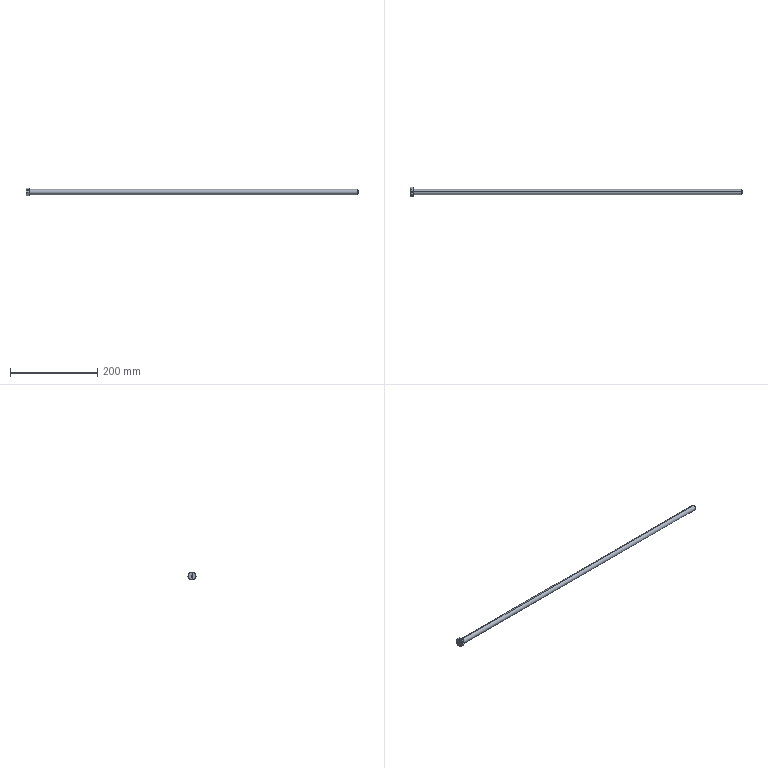Part | SolidWorks | features RevCut 3, CirPattern 1, Cut 1, Extrusion 1, Fillet 1, LPattern 1, Revolution 1 | 1 solid | 32 faces | box 760.5 x 20.785 x 18 mm | volume 86944 mm3 | cylinder 10 | cone 10 | plane 10 | torus 2 | commonest cylinder face diameters 3.2 x8 12 x2
STEP:
#1=CARTESIAN_POINT('',(3.8,8.594,-3.114));
#2=VERTEX_POINT('',#1);
#3=CARTESIAN_POINT('',(3.8,6.994,-5.886));
#4=VERTEX_POINT('',#3);
#5=CARTESIAN_POINT('',(3.8,7.794,-4.5));
#6=DIRECTION('',(0.,-0.866,0.5));
#7=DIRECTION('',(0.,-0.5,-0.866));
#8=AXIS2_PLACEMENT_3D('',#5,#6,#7);
#9=CIRCLE('',#8,1.6);
#10=EDGE_CURVE('',#2,#4,#9,.T.);
#11=ORIENTED_EDGE('',*,*,#10,.F.);
#12=CARTESIAN_POINT('',(3.8,1.6,0.9238));
#13=VERTEX_POINT('',#12);
#14=CARTESIAN_POINT('',(3.8,12.491,-5.364));
#15=DIRECTION('',(0.,-0.866,0.5));
#16=VECTOR('',#15,1000.);
#17=LINE('',#14,#16);
#18=EDGE_CURVE('',#2,#13,#17,.T.);
#19=ORIENTED_EDGE('',*,*,#18,.T.);
#20=CARTESIAN_POINT('',(2.2,0.,0.));
#21=VERTEX_POINT('',#20);
#22=CARTESIAN_POINT('',(2.2,0.,0.));
#23=CARTESIAN_POINT('',(2.2,0.9373,0.5411));
#24=CARTESIAN_POINT('',(2.863,1.6,0.9238));
#25=CARTESIAN_POINT('',(3.8,1.6,0.9238));
#26=(BOUNDED_CURVE()B_SPLINE_CURVE(3,(#22,#23,#24,#25),.UNSPECIFIED.,.F.,.T.)B_SPLINE_CURVE_WITH_KNOTS((4,4),(4.712,6.283),.UNSPECIFIED.)CURVE()GEOMETRIC_REPRESENTATION_ITEM()RATIONAL_B_SPLINE_CURVE((1.,0.8047,0.8047,1.))REPRESENTATION_ITEM(''));
#27=EDGE_CURVE('',#21,#13,#26,.T.);
#28=ORIENTED_EDGE('',*,*,#27,.F.);
#29=CARTESIAN_POINT('',(3.8,1.6,-2.771));
#30=VERTEX_POINT('',#29);
#31=CARTESIAN_POINT('',(3.8,1.6,-2.771));
#32=CARTESIAN_POINT('',(2.863,1.6,-2.771));
#33=CARTESIAN_POINT('',(2.2,0.9373,-1.623));
#34=CARTESIAN_POINT('',(2.2,0.,0.));
#35=(BOUNDED_CURVE()B_SPLINE_CURVE(3,(#31,#32,#33,#34),.UNSPECIFIED.,.F.,.T.)B_SPLINE_CURVE_WITH_KNOTS((4,4),(3.142,4.712),.UNSPECIFIED.)CURVE()GEOMETRIC_REPRESENTATION_ITEM()RATIONAL_B_SPLINE_CURVE((1.,0.8047,0.8047,1.))REPRESENTATION_ITEM(''));
#36=EDGE_CURVE('',#30,#21,#35,.T.);
#37=ORIENTED_EDGE('',*,*,#36,.F.);
#38=CARTESIAN_POINT('',(3.8,10.891,-8.136));
#39=DIRECTION('',(0.,-0.866,0.5));
#40=VECTOR('',#39,1000.);
#41=LINE('',#38,#40);
#42=EDGE_CURVE('',#4,#30,#41,.T.);
#43=ORIENTED_EDGE('',*,*,#42,.F.);
#44=EDGE_LOOP('',(#11,#19,#28,#37,#43));
#45=FACE_OUTER_BOUND('',#44,.T.);
#46=CARTESIAN_POINT('',(3.8,11.691,-6.75));
#47=DIRECTION('',(0.,-0.866,0.5));
#48=DIRECTION('',(0.,-0.5,-0.866));
#49=AXIS2_PLACEMENT_3D('',#46,#47,#48);
#50=CYLINDRICAL_SURFACE('',#49,1.6);
#51=ADVANCED_FACE('',(#45),#50,.F.);
#52=CARTESIAN_POINT('',(3.8,-1.6,2.771));
#53=VERTEX_POINT('',#52);
#54=CARTESIAN_POINT('',(3.8,-1.6,2.771));
#55=CARTESIAN_POINT('',(2.863,-1.6,2.771));
#56=CARTESIAN_POINT('',(2.2,-0.9373,1.623));
#57=CARTESIAN_POINT('',(2.2,0.,0.));
#58=(BOUNDED_CURVE()B_SPLINE_CURVE(3,(#54,#55,#56,#57),.UNSPECIFIED.,.F.,.T.)B_SPLINE_CURVE_WITH_KNOTS((4,4),(0.,1.571),.UNSPECIFIED.)CURVE()GEOMETRIC_REPRESENTATION_ITEM()RATIONAL_B_SPLINE_CURVE((1.,0.8047,0.8047,1.))REPRESENTATION_ITEM(''));
#59=EDGE_CURVE('',#53,#21,#58,.T.);
#60=ORIENTED_EDGE('',*,*,#59,.F.);
#61=CARTESIAN_POINT('',(3.8,-6.994,5.886));
#62=VERTEX_POINT('',#61);
#63=CARTESIAN_POINT('',(3.8,12.491,-5.364));
#64=DIRECTION('',(0.,-0.866,0.5));
#65=VECTOR('',#64,1000.);
#66=LINE('',#63,#65);
#67=EDGE_CURVE('',#53,#62,#66,.T.);
#68=ORIENTED_EDGE('',*,*,#67,.T.);
#69=CARTESIAN_POINT('',(3.8,-8.594,3.114));
#70=VERTEX_POINT('',#69);
#71=CARTESIAN_POINT('',(3.8,-7.794,4.5));
#72=DIRECTION('',(0.,0.866,-0.5));
#73=DIRECTION('',(0.,0.5,0.866));
#74=AXIS2_PLACEMENT_3D('',#71,#72,#73);
#75=CIRCLE('',#74,1.6);
#76=EDGE_CURVE('',#70,#62,#75,.T.);
#77=ORIENTED_EDGE('',*,*,#76,.F.);
#78=CARTESIAN_POINT('',(3.8,-1.6,-0.9238));
#79=VERTEX_POINT('',#78);
#80=CARTESIAN_POINT('',(3.8,10.891,-8.136));
#81=DIRECTION('',(0.,-0.866,0.5));
#82=VECTOR('',#81,1000.);
#83=LINE('',#80,#82);
#84=EDGE_CURVE('',#79,#70,#83,.T.);
#85=ORIENTED_EDGE('',*,*,#84,.F.);
#86=CARTESIAN_POINT('',(2.2,0.,0.));
#87=CARTESIAN_POINT('',(2.2,-0.9373,-0.5411));
#88=CARTESIAN_POINT('',(2.863,-1.6,-0.9238));
#89=CARTESIAN_POINT('',(3.8,-1.6,-0.9238));
#90=(BOUNDED_CURVE()B_SPLINE_CURVE(3,(#86,#87,#88,#89),.UNSPECIFIED.,.F.,.T.)B_SPLINE_CURVE_WITH_KNOTS((4,4),(1.571,3.142),.UNSPECIFIED.)CURVE()GEOMETRIC_REPRESENTATION_ITEM()RATIONAL_B_SPLINE_CURVE((1.,0.8047,0.8047,1.))REPRESENTATION_ITEM(''));
#91=EDGE_CURVE('',#21,#79,#90,.T.);
#92=ORIENTED_EDGE('',*,*,#91,.F.);
#93=EDGE_LOOP('',(#60,#68,#77,#85,#92));
#94=FACE_OUTER_BOUND('',#93,.T.);
#95=CARTESIAN_POINT('',(3.8,11.691,-6.75));
#96=DIRECTION('',(0.,-0.866,0.5));
#97=DIRECTION('',(0.,-0.5,-0.866));
#98=AXIS2_PLACEMENT_3D('',#95,#96,#97);
#99=CYLINDRICAL_SURFACE('',#98,1.6);
#100=ADVANCED_FACE('',(#94),#99,.F.);
#101=CARTESIAN_POINT('',(2.2,0.,-9.));
#102=VERTEX_POINT('',#101);
#103=CARTESIAN_POINT('',(5.4,0.,-9.));
#104=VERTEX_POINT('',#103);
#105=CARTESIAN_POINT('',(3.8,0.,-9.));
#106=DIRECTION('',(0.,0.,1.));
#107=DIRECTION('',(1.,0.,0.));
#108=AXIS2_PLACEMENT_3D('',#105,#106,#107);
#109=CIRCLE('',#108,1.6);
#110=EDGE_CURVE('',#102,#104,#109,.T.);
#111=ORIENTED_EDGE('',*,*,#110,.F.);
#112=CARTESIAN_POINT('',(2.2,0.,-9.));
#113=DIRECTION('',(0.,0.,1.));
#114=VECTOR('',#113,1000.);
#115=LINE('',#112,#114);
#116=EDGE_CURVE('',#102,#21,#115,.T.);
#117=ORIENTED_EDGE('',*,*,#116,.T.);
#118=ORIENTED_EDGE('',*,*,#91,.T.);
#119=CARTESIAN_POINT('',(5.4,0.,0.));
#120=VERTEX_POINT('',#119);
#121=CARTESIAN_POINT('',(3.8,-1.6,-0.9238));
#122=CARTESIAN_POINT('',(4.737,-1.6,-0.9238));
#123=CARTESIAN_POINT('',(5.4,-0.9373,-0.5411));
#124=CARTESIAN_POINT('',(5.4,0.,0.));
#125=(BOUNDED_CURVE()B_SPLINE_CURVE(3,(#121,#122,#123,#124),.UNSPECIFIED.,.F.,.T.)B_SPLINE_CURVE_WITH_KNOTS((4,4),(3.142,4.712),.UNSPECIFIED.)CURVE()GEOMETRIC_REPRESENTATION_ITEM()RATIONAL_B_SPLINE_CURVE((1.,0.8047,0.8047,1.))REPRESENTATION_ITEM(''));
#126=EDGE_CURVE('',#79,#120,#125,.T.);
#127=ORIENTED_EDGE('',*,*,#126,.T.);
#128=CARTESIAN_POINT('',(5.4,0.,-9.));
#129=DIRECTION('',(0.,0.,1.));
#130=VECTOR('',#129,1000.);
#131=LINE('',#128,#130);
#132=EDGE_CURVE('',#104,#120,#131,.T.);
#133=ORIENTED_EDGE('',*,*,#132,.F.);
#134=EDGE_LOOP('',(#111,#117,#118,#127,#133));
#135=FACE_OUTER_BOUND('',#134,.T.);
#136=CARTESIAN_POINT('',(3.8,0.,-9.));
#137=DIRECTION('',(0.,0.,1.));
#138=DIRECTION('',(1.,0.,0.));
#139=AXIS2_PLACEMENT_3D('',#136,#137,#138);
#140=CYLINDRICAL_SURFACE('',#139,1.6);
#141=ADVANCED_FACE('',(#135),#140,.F.);
#142=CARTESIAN_POINT('',(760.5,0.,4.484));
#143=VERTEX_POINT('',#142);
#144=CARTESIAN_POINT('',(760.5,0.,-4.484));
#145=VERTEX_POINT('',#144);
#146=CARTESIAN_POINT('',(760.5,0.,0.));
#147=DIRECTION('',(-1.,0.,0.));
#148=DIRECTION('',(0.,0.,1.));
#149=AXIS2_PLACEMENT_3D('',#146,#147,#148);
#150=CIRCLE('',#149,4.484);
#151=EDGE_CURVE('',#143,#145,#150,.T.);
#152=ORIENTED_EDGE('',*,*,#151,.T.);
#153=CARTESIAN_POINT('',(759.625,0.,-6.));
#154=VERTEX_POINT('',#153);
#155=CARTESIAN_POINT('',(759.625,0.,-6.));
#156=DIRECTION('',(-0.5,0.,-0.866));
#157=VECTOR('',#156,1000.);
#158=LINE('',#155,#157);
#159=EDGE_CURVE('',#145,#154,#158,.T.);
#160=ORIENTED_EDGE('',*,*,#159,.T.);
#161=CARTESIAN_POINT('',(759.625,0.,6.));
#162=VERTEX_POINT('',#161);
#163=CARTESIAN_POINT('',(759.625,0.,0.));
#164=DIRECTION('',(-1.,0.,0.));
#165=DIRECTION('',(0.,0.,1.));
#166=AXIS2_PLACEMENT_3D('',#163,#164,#165);
#167=CIRCLE('',#166,6.);
#168=EDGE_CURVE('',#162,#154,#167,.T.);
#169=ORIENTED_EDGE('',*,*,#168,.F.);
#170=CARTESIAN_POINT('',(759.625,0.,6.));
#171=DIRECTION('',(-0.5,0.,0.866));
#172=VECTOR('',#171,1000.);
#173=LINE('',#170,#172);
#174=EDGE_CURVE('',#143,#162,#173,.T.);
#175=ORIENTED_EDGE('',*,*,#174,.F.);
#176=EDGE_LOOP('',(#152,#160,#169,#175));
#177=FACE_OUTER_BOUND('',#176,.T.);
#178=CARTESIAN_POINT('',(759.625,0.,0.));
#179=DIRECTION('',(-1.,0.,0.));
#180=DIRECTION('',(0.,0.,1.));
#181=AXIS2_PLACEMENT_3D('',#178,#179,#180);
#182=CONICAL_SURFACE('',#181,6.,1.047);
#183=ADVANCED_FACE('',(#177),#182,.T.);
#184=CARTESIAN_POINT('',(8.1,0.,6.));
#185=VERTEX_POINT('',#184);
#186=CARTESIAN_POINT('',(8.1,0.,-6.));
#187=VERTEX_POINT('',#186);
#188=CARTESIAN_POINT('',(8.1,0.,0.));
#189=DIRECTION('',(1.,0.,0.));
#190=DIRECTION('',(0.,0.,-1.));
#191=AXIS2_PLACEMENT_3D('',#188,#189,#190);
#192=CIRCLE('',#191,6.);
#193=EDGE_CURVE('',#185,#187,#192,.T.);
#194=ORIENTED_EDGE('',*,*,#193,.F.);
#195=CARTESIAN_POINT('',(7.5,0.,6.6));
#196=VERTEX_POINT('',#195);
#197=CARTESIAN_POINT('',(8.1,0.,6.6));
#198=DIRECTION('',(0.,1.,0.));
#199=DIRECTION('',(0.,0.,1.));
#200=AXIS2_PLACEMENT_3D('',#197,#198,#199);
#201=CIRCLE('',#200,0.6);
#202=EDGE_CURVE('',#185,#196,#201,.T.);
#203=ORIENTED_EDGE('',*,*,#202,.T.);
#204=CARTESIAN_POINT('',(7.5,0.,-6.6));
#205=VERTEX_POINT('',#204);
#206=CARTESIAN_POINT('',(7.5,0.,0.));
#207=DIRECTION('',(-1.,0.,0.));
#208=DIRECTION('',(0.,0.,-1.));
#209=AXIS2_PLACEMENT_3D('',#206,#207,#208);
#210=CIRCLE('',#209,6.6);
#211=EDGE_CURVE('',#205,#196,#210,.T.);
#212=ORIENTED_EDGE('',*,*,#211,.F.);
#213=CARTESIAN_POINT('',(8.1,0.,-6.6));
#214=DIRECTION('',(0.,-1.,0.));
#215=DIRECTION('',(0.,0.,-1.));
#216=AXIS2_PLACEMENT_3D('',#213,#214,#215);
#217=CIRCLE('',#216,0.6);
#218=EDGE_CURVE('',#187,#205,#217,.T.);
#219=ORIENTED_EDGE('',*,*,#218,.F.);
#220=EDGE_LOOP('',(#194,#203,#212,#219));
#221=FACE_OUTER_BOUND('',#220,.T.);
#222=CARTESIAN_POINT('',(8.1,0.,0.));
#223=DIRECTION('',(1.,0.,0.));
#224=DIRECTION('',(0.,0.,-1.));
#225=AXIS2_PLACEMENT_3D('',#222,#223,#224);
#226=TOROIDAL_SURFACE('',#225,6.6,0.6);
#227=ADVANCED_FACE('',(#221),#226,.F.);
#228=CARTESIAN_POINT('',(7.5,-8.315,0.));
#229=VERTEX_POINT('',#228);
#230=CARTESIAN_POINT('',(7.5,8.315,0.));
#231=VERTEX_POINT('',#230);
#232=CARTESIAN_POINT('',(7.5,0.,0.));
#233=DIRECTION('',(-1.,0.,0.));
#234=DIRECTION('',(0.,-1.,0.));
#235=AXIS2_PLACEMENT_3D('',#232,#233,#234);
#236=CIRCLE('',#235,8.315);
#237=EDGE_CURVE('',#229,#231,#236,.T.);
#238=ORIENTED_EDGE('',*,*,#237,.T.);
#239=CARTESIAN_POINT('',(6.9,8.661,0.));
#240=VERTEX_POINT('',#239);
#241=CARTESIAN_POINT('',(6.9,8.661,0.));
#242=DIRECTION('',(-0.866,0.5,0.));
#243=VECTOR('',#242,1000.);
#244=LINE('',#241,#243);
#245=EDGE_CURVE('',#231,#240,#244,.T.);
#246=ORIENTED_EDGE('',*,*,#245,.T.);
#247=CARTESIAN_POINT('',(6.9,-8.661,0.));
#248=VERTEX_POINT('',#247);
#249=CARTESIAN_POINT('',(6.9,0.,0.));
#250=DIRECTION('',(-1.,0.,0.));
#251=DIRECTION('',(0.,-1.,0.));
#252=AXIS2_PLACEMENT_3D('',#249,#250,#251);
#253=CIRCLE('',#252,8.661);
#254=EDGE_CURVE('',#248,#240,#253,.T.);
#255=ORIENTED_EDGE('',*,*,#254,.F.);
#256=CARTESIAN_POINT('',(6.9,-8.661,0.));
#257=DIRECTION('',(-0.866,-0.5,0.));
#258=VECTOR('',#257,1000.);
#259=LINE('',#256,#258);
#260=EDGE_CURVE('',#229,#248,#259,.T.);
#261=ORIENTED_EDGE('',*,*,#260,.F.);
#262=EDGE_LOOP('',(#238,#246,#255,#261));
#263=FACE_OUTER_BOUND('',#262,.T.);
#264=CARTESIAN_POINT('',(6.9,0.,0.));
#265=DIRECTION('',(-1.,0.,0.));
#266=DIRECTION('',(0.,-1.,0.));
#267=AXIS2_PLACEMENT_3D('',#264,#265,#266);
#268=CONICAL_SURFACE('',#267,8.661,0.5236);
#269=ADVANCED_FACE('',(#263),#268,.T.);
#270=ORIENTED_EDGE('',*,*,#168,.T.);
#271=CARTESIAN_POINT('',(0.,0.,-6.));
#272=DIRECTION('',(-1.,0.,0.));
#273=VECTOR('',#272,1000.);
#274=LINE('',#271,#273);
#275=EDGE_CURVE('',#154,#187,#274,.T.);
#276=ORIENTED_EDGE('',*,*,#275,.T.);
#277=CARTESIAN_POINT('',(8.1,0.,0.));
#278=DIRECTION('',(1.,0.,0.));
#279=DIRECTION('',(0.,0.,-1.));
#280=AXIS2_PLACEMENT_3D('',#277,#278,#279);
#281=CIRCLE('',#280,6.);
#282=EDGE_CURVE('',#187,#185,#281,.T.);
#283=ORIENTED_EDGE('',*,*,#282,.T.);
#284=CARTESIAN_POINT('',(0.,0.,6.));
#285=DIRECTION('',(-1.,0.,0.));
#286=VECTOR('',#285,1000.);
#287=LINE('',#284,#286);
#288=EDGE_CURVE('',#162,#185,#287,.T.);
#289=ORIENTED_EDGE('',*,*,#288,.F.);
#290=EDGE_LOOP('',(#270,#276,#283,#289));
#291=FACE_OUTER_BOUND('',#290,.T.);
#292=CARTESIAN_POINT('',(0.,0.,0.));
#293=DIRECTION('',(-1.,0.,0.));
#294=DIRECTION('',(0.,0.,1.));
#295=AXIS2_PLACEMENT_3D('',#292,#293,#294);
#296=CYLINDRICAL_SURFACE('',#295,6.);
#297=ADVANCED_FACE('',(#291),#296,.T.);
#298=CARTESIAN_POINT('',(5.4,0.,0.));
#299=CARTESIAN_POINT('',(5.4,-0.9373,1.623));
#300=CARTESIAN_POINT('',(4.737,-1.6,2.771));
#301=CARTESIAN_POINT('',(3.8,-1.6,2.771));
#302=(BOUNDED_CURVE()B_SPLINE_CURVE(3,(#298,#299,#300,#301),.UNSPECIFIED.,.F.,.T.)B_SPLINE_CURVE_WITH_KNOTS((4,4),(4.712,6.283),.UNSPECIFIED.)CURVE()GEOMETRIC_REPRESENTATION_ITEM()RATIONAL_B_SPLINE_CURVE((1.,0.8047,0.8047,1.))REPRESENTATION_ITEM(''));
#303=EDGE_CURVE('',#120,#53,#302,.T.);
#304=ORIENTED_EDGE('',*,*,#303,.T.);
#305=ORIENTED_EDGE('',*,*,#59,.T.);
#306=CARTESIAN_POINT('',(2.2,0.,9.));
#307=VERTEX_POINT('',#306);
#308=CARTESIAN_POINT('',(2.2,0.,-9.));
#309=DIRECTION('',(0.,0.,1.));
#310=VECTOR('',#309,1000.);
#311=LINE('',#308,#310);
#312=EDGE_CURVE('',#21,#307,#311,.T.);
#313=ORIENTED_EDGE('',*,*,#312,.T.);
#314=CARTESIAN_POINT('',(5.4,0.,9.));
#315=VERTEX_POINT('',#314);
#316=CARTESIAN_POINT('',(3.8,0.,9.));
#317=DIRECTION('',(0.,0.,1.));
#318=DIRECTION('',(1.,0.,0.));
#319=AXIS2_PLACEMENT_3D('',#316,#317,#318);
#320=CIRCLE('',#319,1.6);
#321=EDGE_CURVE('',#307,#315,#320,.T.);
#322=ORIENTED_EDGE('',*,*,#321,.T.);
#323=CARTESIAN_POINT('',(5.4,0.,-9.));
#324=DIRECTION('',(0.,0.,1.));
#325=VECTOR('',#324,1000.);
#326=LINE('',#323,#325);
#327=EDGE_CURVE('',#120,#315,#326,.T.);
#328=ORIENTED_EDGE('',*,*,#327,.F.);
#329=EDGE_LOOP('',(#304,#305,#313,#322,#328));
#330=FACE_OUTER_BOUND('',#329,.T.);
#331=CARTESIAN_POINT('',(3.8,0.,-9.));
#332=DIRECTION('',(0.,0.,1.));
#333=DIRECTION('',(1.,0.,0.));
#334=AXIS2_PLACEMENT_3D('',#331,#332,#333);
#335=CYLINDRICAL_SURFACE('',#334,1.6);
#336=ADVANCED_FACE('',(#330),#335,.F.);
#337=ORIENTED_EDGE('',*,*,#312,.F.);
#338=ORIENTED_EDGE('',*,*,#27,.T.);
#339=CARTESIAN_POINT('',(3.8,1.6,0.9238));
#340=CARTESIAN_POINT('',(4.737,1.6,0.9238));
#341=CARTESIAN_POINT('',(5.4,0.9373,0.5411));
#342=CARTESIAN_POINT('',(5.4,0.,0.));
#343=(BOUNDED_CURVE()B_SPLINE_CURVE(3,(#339,#340,#341,#342),.UNSPECIFIED.,.F.,.T.)B_SPLINE_CURVE_WITH_KNOTS((4,4),(0.,1.571),.UNSPECIFIED.)CURVE()GEOMETRIC_REPRESENTATION_ITEM()RATIONAL_B_SPLINE_CURVE((1.,0.8047,0.8047,1.))REPRESENTATION_ITEM(''));
#344=EDGE_CURVE('',#13,#120,#343,.T.);
#345=ORIENTED_EDGE('',*,*,#344,.T.);
#346=ORIENTED_EDGE('',*,*,#327,.T.);
#347=CARTESIAN_POINT('',(3.8,0.,9.));
#348=DIRECTION('',(0.,0.,1.));
#349=DIRECTION('',(1.,0.,0.));
#350=AXIS2_PLACEMENT_3D('',#347,#348,#349);
#351=CIRCLE('',#350,1.6);
#352=EDGE_CURVE('',#315,#307,#351,.T.);
#353=ORIENTED_EDGE('',*,*,#352,.T.);
#354=EDGE_LOOP('',(#337,#338,#345,#346,#353));
#355=FACE_OUTER_BOUND('',#354,.T.);
#356=CARTESIAN_POINT('',(3.8,0.,-9.));
#357=DIRECTION('',(0.,0.,1.));
#358=DIRECTION('',(1.,0.,0.));
#359=AXIS2_PLACEMENT_3D('',#356,#357,#358);
#360=CYLINDRICAL_SURFACE('',#359,1.6);
#361=ADVANCED_FACE('',(#355),#360,.F.);
#362=ORIENTED_EDGE('',*,*,#275,.F.);
#363=CARTESIAN_POINT('',(759.625,0.,0.));
#364=DIRECTION('',(-1.,0.,0.));
#365=DIRECTION('',(0.,0.,1.));
#366=AXIS2_PLACEMENT_3D('',#363,#364,#365);
#367=CIRCLE('',#366,6.);
#368=EDGE_CURVE('',#154,#162,#367,.T.);
#369=ORIENTED_EDGE('',*,*,#368,.T.);
#370=ORIENTED_EDGE('',*,*,#288,.T.);
#371=ORIENTED_EDGE('',*,*,#193,.T.);
#372=EDGE_LOOP('',(#362,#369,#370,#371));
#373=FACE_OUTER_BOUND('',#372,.T.);
#374=CARTESIAN_POINT('',(0.,0.,0.));
#375=DIRECTION('',(-1.,0.,0.));
#376=DIRECTION('',(0.,0.,1.));
#377=AXIS2_PLACEMENT_3D('',#374,#375,#376);
#378=CYLINDRICAL_SURFACE('',#377,6.);
#379=ADVANCED_FACE('',(#373),#378,.T.);
#380=CARTESIAN_POINT('',(3.8,7.794,-4.5));
#381=DIRECTION('',(0.,-0.866,0.5));
#382=DIRECTION('',(0.,-0.5,-0.866));
#383=AXIS2_PLACEMENT_3D('',#380,#381,#382);
#384=CIRCLE('',#383,1.6);
#385=EDGE_CURVE('',#4,#2,#384,.T.);
#386=ORIENTED_EDGE('',*,*,#385,.T.);
#387=ORIENTED_EDGE('',*,*,#10,.T.);
#388=EDGE_LOOP('',(#386,#387));
#389=FACE_BOUND('',#388,.T.);
#390=CARTESIAN_POINT('',(6.9,5.196,-9.));
#391=VERTEX_POINT('',#390);
#392=CARTESIAN_POINT('',(6.9,10.392,0.));
#393=VERTEX_POINT('',#392);
#394=CARTESIAN_POINT('',(6.9,5.196,-9.));
#395=DIRECTION('',(0.,0.5,0.866));
#396=VECTOR('',#395,1000.);
#397=LINE('',#394,#396);
#398=EDGE_CURVE('',#391,#393,#397,.T.);
#399=ORIENTED_EDGE('',*,*,#398,.F.);
#400=CARTESIAN_POINT('',(0.8038,5.196,-9.));
#401=VERTEX_POINT('',#400);
#402=CARTESIAN_POINT('',(7.5,5.196,-9.));
#403=DIRECTION('',(-1.,0.,0.));
#404=VECTOR('',#403,1000.);
#405=LINE('',#402,#404);
#406=EDGE_CURVE('',#391,#401,#405,.T.);
#407=ORIENTED_EDGE('',*,*,#406,.T.);
#408=CARTESIAN_POINT('',(0.,7.794,-4.5));
#409=VERTEX_POINT('',#408);
#410=CARTESIAN_POINT('',(0.,7.794,-4.5));
#411=CARTESIAN_POINT('',(0.,7.574,-4.882));
#412=CARTESIAN_POINT('',(0.019,7.352,-5.266));
#413=CARTESIAN_POINT('',(0.09253,6.914,-6.024));
#414=CARTESIAN_POINT('',(0.147,6.697,-6.401));
#415=CARTESIAN_POINT('',(0.357,6.048,-7.525));
#416=CARTESIAN_POINT('',(0.5591,5.62,-8.266));
#417=CARTESIAN_POINT('',(0.8038,5.196,-9.));
#418=B_SPLINE_CURVE_WITH_KNOTS('',3,(#410,#411,#412,#413,#414,#415,#416,#417),.UNSPECIFIED.,.F.,.F.,(4,2,2,4),(0.005258,0.006567,0.007877,0.0105),.UNSPECIFIED.);
#419=EDGE_CURVE('',#409,#401,#418,.T.);
#420=ORIENTED_EDGE('',*,*,#419,.F.);
#421=CARTESIAN_POINT('',(0.8038,10.392,0.));
#422=VERTEX_POINT('',#421);
#423=CARTESIAN_POINT('',(0.8038,10.392,0.));
#424=CARTESIAN_POINT('',(0.5585,9.967,-0.7361));
#425=CARTESIAN_POINT('',(0.3563,9.539,-1.478));
#426=CARTESIAN_POINT('',(0.07661,8.674,-2.976));
#427=CARTESIAN_POINT('',(0.,8.237,-3.733));
#428=CARTESIAN_POINT('',(0.,7.794,-4.5));
#429=B_SPLINE_CURVE_WITH_KNOTS('',3,(#423,#424,#425,#426,#427,#428),.UNSPECIFIED.,.F.,.F.,(4,2,4),(0.000000238,0.002629,0.005258),.UNSPECIFIED.);
#430=EDGE_CURVE('',#422,#409,#429,.T.);
#431=ORIENTED_EDGE('',*,*,#430,.F.);
#432=CARTESIAN_POINT('',(7.5,10.392,0.));
#433=DIRECTION('',(-1.,0.,0.));
#434=VECTOR('',#433,1000.);
#435=LINE('',#432,#434);
#436=EDGE_CURVE('',#393,#422,#435,.T.);
#437=ORIENTED_EDGE('',*,*,#436,.F.);
#438=EDGE_LOOP('',(#399,#407,#420,#431,#437));
#439=FACE_OUTER_BOUND('',#438,.T.);
#440=CARTESIAN_POINT('',(7.5,5.196,-9.));
#441=DIRECTION('',(0.,-0.866,0.5));
#442=DIRECTION('',(0.,-0.5,-0.866));
#443=AXIS2_PLACEMENT_3D('',#440,#441,#442);
#444=PLANE('',#443);
#445=ADVANCED_FACE('',(#389,#439),#444,.F.);
#446=CARTESIAN_POINT('',(6.9,5.196,9.));
#447=VERTEX_POINT('',#446);
#448=CARTESIAN_POINT('',(6.9,10.392,0.));
#449=DIRECTION('',(0.,-0.5,0.866));
#450=VECTOR('',#449,1000.);
#451=LINE('',#448,#450);
#452=EDGE_CURVE('',#393,#447,#451,.T.);
#453=ORIENTED_EDGE('',*,*,#452,.F.);
#454=ORIENTED_EDGE('',*,*,#436,.T.);
#455=CARTESIAN_POINT('',(0.,7.794,4.5));
#456=VERTEX_POINT('',#455);
#457=CARTESIAN_POINT('',(0.,7.794,4.5));
#458=CARTESIAN_POINT('',(0.,8.015,4.118));
#459=CARTESIAN_POINT('',(0.019,8.236,3.734));
#460=CARTESIAN_POINT('',(0.09253,8.674,2.976));
#461=CARTESIAN_POINT('',(0.147,8.892,2.599));
#462=CARTESIAN_POINT('',(0.357,9.541,1.475));
#463=CARTESIAN_POINT('',(0.5591,9.968,0.7343));
#464=CARTESIAN_POINT('',(0.8038,10.392,0.));
#465=B_SPLINE_CURVE_WITH_KNOTS('',3,(#457,#458,#459,#460,#461,#462,#463,#464),.UNSPECIFIED.,.F.,.F.,(4,2,2,4),(0.005258,0.006567,0.007877,0.0105),.UNSPECIFIED.);
#466=EDGE_CURVE('',#456,#422,#465,.T.);
#467=ORIENTED_EDGE('',*,*,#466,.F.);
#468=CARTESIAN_POINT('',(0.8038,5.196,9.));
#469=VERTEX_POINT('',#468);
#470=CARTESIAN_POINT('',(0.8038,5.196,9.));
#471=CARTESIAN_POINT('',(0.5585,5.621,8.264));
#472=CARTESIAN_POINT('',(0.3563,6.049,7.522));
#473=CARTESIAN_POINT('',(0.07661,6.914,6.024));
#474=CARTESIAN_POINT('',(0.,7.352,5.267));
#475=CARTESIAN_POINT('',(0.,7.794,4.5));
#476=B_SPLINE_CURVE_WITH_KNOTS('',3,(#470,#471,#472,#473,#474,#475),.UNSPECIFIED.,.F.,.F.,(4,2,4),(0.000000238,0.002629,0.005258),.UNSPECIFIED.);
#477=EDGE_CURVE('',#469,#456,#476,.T.);
#478=ORIENTED_EDGE('',*,*,#477,.F.);
#479=CARTESIAN_POINT('',(7.5,5.196,9.));
#480=DIRECTION('',(-1.,0.,0.));
#481=VECTOR('',#480,1000.);
#482=LINE('',#479,#481);
#483=EDGE_CURVE('',#447,#469,#482,.T.);
#484=ORIENTED_EDGE('',*,*,#483,.F.);
#485=EDGE_LOOP('',(#453,#454,#467,#478,#484));
#486=FACE_OUTER_BOUND('',#485,.T.);
#487=CARTESIAN_POINT('',(7.5,10.392,0.));
#488=DIRECTION('',(0.,-0.866,-0.5));
#489=DIRECTION('',(0.,0.5,-0.866));
#490=AXIS2_PLACEMENT_3D('',#487,#488,#489);
#491=PLANE('',#490);
#492=ADVANCED_FACE('',(#486),#491,.F.);
#493=ORIENTED_EDGE('',*,*,#352,.F.);
#494=ORIENTED_EDGE('',*,*,#321,.F.);
#495=EDGE_LOOP('',(#493,#494));
#496=FACE_BOUND('',#495,.T.);
#497=CARTESIAN_POINT('',(6.9,-5.196,9.));
#498=VERTEX_POINT('',#497);
#499=CARTESIAN_POINT('',(6.9,5.196,9.));
#500=DIRECTION('',(0.,-1.,0.));
#501=VECTOR('',#500,1000.);
#502=LINE('',#499,#501);
#503=EDGE_CURVE('',#447,#498,#502,.T.);
#504=ORIENTED_EDGE('',*,*,#503,.F.);
#505=ORIENTED_EDGE('',*,*,#483,.T.);
#506=CARTESIAN_POINT('',(0.,0.,9.));
#507=VERTEX_POINT('',#506);
#508=CARTESIAN_POINT('',(0.,0.,9.));
#509=CARTESIAN_POINT('',(0.,0.4401,9.));
#510=CARTESIAN_POINT('',(0.01885,0.8832,9.));
#511=CARTESIAN_POINT('',(0.09319,1.767,9.));
#512=CARTESIAN_POINT('',(0.1482,2.204,9.));
#513=CARTESIAN_POINT('',(0.3593,3.505,9.));
#514=CARTESIAN_POINT('',(0.5612,4.356,9.));
#515=CARTESIAN_POINT('',(0.8038,5.196,9.));
#516=B_SPLINE_CURVE_WITH_KNOTS('',3,(#508,#509,#510,#511,#512,#513,#514,#515),.UNSPECIFIED.,.F.,.F.,(4,2,2,4),(0.01498,0.0163,0.01761,0.02025),.UNSPECIFIED.);
#517=EDGE_CURVE('',#507,#469,#516,.T.);
#518=ORIENTED_EDGE('',*,*,#517,.F.);
#519=CARTESIAN_POINT('',(0.8038,-5.196,9.));
#520=VERTEX_POINT('',#519);
#521=CARTESIAN_POINT('',(0.8038,-5.196,9.));
#522=CARTESIAN_POINT('',(0.5595,-4.35,9.));
#523=CARTESIAN_POINT('',(0.3552,-3.485,9.));
#524=CARTESIAN_POINT('',(0.07569,-1.752,9.));
#525=CARTESIAN_POINT('',(0.,-0.8794,9.));
#526=CARTESIAN_POINT('',(0.,0.,9.));
#527=B_SPLINE_CURVE_WITH_KNOTS('',3,(#521,#522,#523,#524,#525,#526),.UNSPECIFIED.,.F.,.F.,(4,2,4),(0.00972,0.01235,0.01498),.UNSPECIFIED.);
#528=EDGE_CURVE('',#520,#507,#527,.T.);
#529=ORIENTED_EDGE('',*,*,#528,.F.);
#530=CARTESIAN_POINT('',(7.5,-5.196,9.));
#531=DIRECTION('',(-1.,0.,0.));
#532=VECTOR('',#531,1000.);
#533=LINE('',#530,#532);
#534=EDGE_CURVE('',#498,#520,#533,.T.);
#535=ORIENTED_EDGE('',*,*,#534,.F.);
#536=EDGE_LOOP('',(#504,#505,#518,#529,#535));
#537=FACE_OUTER_BOUND('',#536,.T.);
#538=CARTESIAN_POINT('',(7.5,5.196,9.));
#539=DIRECTION('',(0.,0.,-1.));
#540=DIRECTION('',(0.,1.,0.));
#541=AXIS2_PLACEMENT_3D('',#538,#539,#540);
#542=PLANE('',#541);
#543=ADVANCED_FACE('',(#496,#537),#542,.F.);
#544=ORIENTED_EDGE('',*,*,#76,.T.);
#545=CARTESIAN_POINT('',(3.8,-7.794,4.5));
#546=DIRECTION('',(0.,0.866,-0.5));
#547=DIRECTION('',(0.,0.5,0.866));
#548=AXIS2_PLACEMENT_3D('',#545,#546,#547);
#549=CIRCLE('',#548,1.6);
#550=EDGE_CURVE('',#62,#70,#549,.T.);
#551=ORIENTED_EDGE('',*,*,#550,.T.);
#552=EDGE_LOOP('',(#544,#551));
#553=FACE_BOUND('',#552,.T.);
#554=CARTESIAN_POINT('',(6.9,-10.392,0.));
#555=VERTEX_POINT('',#554);
#556=CARTESIAN_POINT('',(6.9,-10.392,0.));
#557=DIRECTION('',(0.,-0.5,-0.866));
#558=VECTOR('',#557,1000.);
#559=LINE('',#556,#558);
#560=EDGE_CURVE('',#498,#555,#559,.T.);
#561=ORIENTED_EDGE('',*,*,#560,.F.);
#562=ORIENTED_EDGE('',*,*,#534,.T.);
#563=CARTESIAN_POINT('',(0.,-7.794,4.5));
#564=VERTEX_POINT('',#563);
#565=CARTESIAN_POINT('',(0.,-7.794,4.5));
#566=CARTESIAN_POINT('',(0.,-7.574,4.882));
#567=CARTESIAN_POINT('',(0.019,-7.352,5.266));
#568=CARTESIAN_POINT('',(0.09253,-6.914,6.024));
#569=CARTESIAN_POINT('',(0.147,-6.697,6.401));
#570=CARTESIAN_POINT('',(0.357,-6.048,7.525));
#571=CARTESIAN_POINT('',(0.5591,-5.62,8.266));
#572=CARTESIAN_POINT('',(0.8038,-5.196,9.));
#573=B_SPLINE_CURVE_WITH_KNOTS('',3,(#565,#566,#567,#568,#569,#570,#571,#572),.UNSPECIFIED.,.F.,.F.,(4,2,2,4),(0.005258,0.006567,0.007877,0.0105),.UNSPECIFIED.);
#574=EDGE_CURVE('',#564,#520,#573,.T.);
#575=ORIENTED_EDGE('',*,*,#574,.F.);
#576=CARTESIAN_POINT('',(0.8038,-10.392,0.));
#577=VERTEX_POINT('',#576);
#578=CARTESIAN_POINT('',(0.8038,-10.392,0.));
#579=CARTESIAN_POINT('',(0.5585,-9.967,0.7361));
#580=CARTESIAN_POINT('',(0.3563,-9.539,1.478));
#581=CARTESIAN_POINT('',(0.07661,-8.674,2.976));
#582=CARTESIAN_POINT('',(0.,-8.237,3.733));
#583=CARTESIAN_POINT('',(0.,-7.794,4.5));
#584=B_SPLINE_CURVE_WITH_KNOTS('',3,(#578,#579,#580,#581,#582,#583),.UNSPECIFIED.,.F.,.F.,(4,2,4),(0.000000238,0.002629,0.005258),.UNSPECIFIED.);
#585=EDGE_CURVE('',#577,#564,#584,.T.);
#586=ORIENTED_EDGE('',*,*,#585,.F.);
#587=CARTESIAN_POINT('',(7.5,-10.392,0.));
#588=DIRECTION('',(-1.,0.,0.));
#589=VECTOR('',#588,1000.);
#590=LINE('',#587,#589);
#591=EDGE_CURVE('',#555,#577,#590,.T.);
#592=ORIENTED_EDGE('',*,*,#591,.F.);
#593=EDGE_LOOP('',(#561,#562,#575,#586,#592));
#594=FACE_OUTER_BOUND('',#593,.T.);
#595=CARTESIAN_POINT('',(7.5,-10.392,0.));
#596=DIRECTION('',(0.,0.866,-0.5));
#597=DIRECTION('',(0.,0.5,0.866));
#598=AXIS2_PLACEMENT_3D('',#595,#596,#597);
#599=PLANE('',#598);
#600=ADVANCED_FACE('',(#553,#594),#599,.F.);
#601=CARTESIAN_POINT('',(6.9,-5.196,-9.));
#602=VERTEX_POINT('',#601);
#603=CARTESIAN_POINT('',(6.9,-5.196,-9.));
#604=DIRECTION('',(0.,0.5,-0.866));
#605=VECTOR('',#604,1000.);
#606=LINE('',#603,#605);
#607=EDGE_CURVE('',#555,#602,#606,.T.);
#608=ORIENTED_EDGE('',*,*,#607,.F.);
#609=ORIENTED_EDGE('',*,*,#591,.T.);
#610=CARTESIAN_POINT('',(0.,-7.794,-4.5));
#611=VERTEX_POINT('',#610);
#612=CARTESIAN_POINT('',(0.,-7.794,-4.5));
#613=CARTESIAN_POINT('',(0.,-8.015,-4.118));
#614=CARTESIAN_POINT('',(0.019,-8.236,-3.734));
#615=CARTESIAN_POINT('',(0.09253,-8.674,-2.976));
#616=CARTESIAN_POINT('',(0.147,-8.892,-2.599));
#617=CARTESIAN_POINT('',(0.357,-9.541,-1.475));
#618=CARTESIAN_POINT('',(0.5591,-9.968,-0.7343));
#619=CARTESIAN_POINT('',(0.8038,-10.392,0.));
#620=B_SPLINE_CURVE_WITH_KNOTS('',3,(#612,#613,#614,#615,#616,#617,#618,#619),.UNSPECIFIED.,.F.,.F.,(4,2,2,4),(0.005258,0.006567,0.007877,0.0105),.UNSPECIFIED.);
#621=EDGE_CURVE('',#611,#577,#620,.T.);
#622=ORIENTED_EDGE('',*,*,#621,.F.);
#623=CARTESIAN_POINT('',(0.8038,-5.196,-9.));
#624=VERTEX_POINT('',#623);
#625=CARTESIAN_POINT('',(0.8038,-5.196,-9.));
#626=CARTESIAN_POINT('',(0.5585,-5.621,-8.264));
#627=CARTESIAN_POINT('',(0.3563,-6.049,-7.522));
#628=CARTESIAN_POINT('',(0.07661,-6.914,-6.024));
#629=CARTESIAN_POINT('',(0.,-7.352,-5.267));
#630=CARTESIAN_POINT('',(0.,-7.794,-4.5));
#631=B_SPLINE_CURVE_WITH_KNOTS('',3,(#625,#626,#627,#628,#629,#630),.UNSPECIFIED.,.F.,.F.,(4,2,4),(0.000000238,0.002629,0.005258),.UNSPECIFIED.);
#632=EDGE_CURVE('',#624,#611,#631,.T.);
#633=ORIENTED_EDGE('',*,*,#632,.F.);
#634=CARTESIAN_POINT('',(7.5,-5.196,-9.));
#635=DIRECTION('',(-1.,0.,0.));
#636=VECTOR('',#635,1000.);
#637=LINE('',#634,#636);
#638=EDGE_CURVE('',#602,#624,#637,.T.);
#639=ORIENTED_EDGE('',*,*,#638,.F.);
#640=EDGE_LOOP('',(#608,#609,#622,#633,#639));
#641=FACE_OUTER_BOUND('',#640,.T.);
#642=CARTESIAN_POINT('',(7.5,-5.196,-9.));
#643=DIRECTION('',(0.,0.866,0.5));
#644=DIRECTION('',(0.,-0.5,0.866));
#645=AXIS2_PLACEMENT_3D('',#642,#643,#644);
#646=PLANE('',#645);
#647=ADVANCED_FACE('',(#641),#646,.F.);
#648=CARTESIAN_POINT('',(3.8,0.,-9.));
#649=DIRECTION('',(0.,0.,1.));
#650=DIRECTION('',(1.,0.,0.));
#651=AXIS2_PLACEMENT_3D('',#648,#649,#650);
#652=CIRCLE('',#651,1.6);
#653=EDGE_CURVE('',#104,#102,#652,.T.);
#654=ORIENTED_EDGE('',*,*,#653,.T.);
#655=ORIENTED_EDGE('',*,*,#110,.T.);
#656=EDGE_LOOP('',(#654,#655));
#657=FACE_BOUND('',#656,.T.);
#658=CARTESIAN_POINT('',(6.9,5.196,-9.));
#659=DIRECTION('',(0.,1.,0.));
#660=VECTOR('',#659,1000.);
#661=LINE('',#658,#660);
#662=EDGE_CURVE('',#602,#391,#661,.T.);
#663=ORIENTED_EDGE('',*,*,#662,.F.);
#664=ORIENTED_EDGE('',*,*,#638,.T.);
#665=CARTESIAN_POINT('',(0.,0.,-9.));
#666=VERTEX_POINT('',#665);
#667=CARTESIAN_POINT('',(0.,0.,-9.));
#668=CARTESIAN_POINT('',(0.,-0.8794,-9.));
#669=CARTESIAN_POINT('',(0.07569,-1.752,-9.));
#670=CARTESIAN_POINT('',(0.3552,-3.485,-9.));
#671=CARTESIAN_POINT('',(0.5595,-4.35,-9.));
#672=CARTESIAN_POINT('',(0.8038,-5.196,-9.));
#673=B_SPLINE_CURVE_WITH_KNOTS('',3,(#667,#668,#669,#670,#671,#672),.UNSPECIFIED.,.F.,.F.,(4,2,4),(0.03045,0.03308,0.03571),.UNSPECIFIED.);
#674=EDGE_CURVE('',#666,#624,#673,.T.);
#675=ORIENTED_EDGE('',*,*,#674,.F.);
#676=CARTESIAN_POINT('',(0.8038,5.196,-9.));
#677=CARTESIAN_POINT('',(0.5612,4.356,-9.));
#678=CARTESIAN_POINT('',(0.3593,3.505,-9.));
#679=CARTESIAN_POINT('',(0.1482,2.204,-9.));
#680=CARTESIAN_POINT('',(0.09319,1.767,-9.));
#681=CARTESIAN_POINT('',(0.01885,0.8832,-9.));
#682=CARTESIAN_POINT('',(0.,0.4401,-9.));
#683=CARTESIAN_POINT('',(0.,0.,-9.));
#684=B_SPLINE_CURVE_WITH_KNOTS('',3,(#676,#677,#678,#679,#680,#681,#682,#683),.UNSPECIFIED.,.F.,.F.,(4,2,2,4),(0.02519,0.02782,0.02914,0.03045),.UNSPECIFIED.);
#685=EDGE_CURVE('',#401,#666,#684,.T.);
#686=ORIENTED_EDGE('',*,*,#685,.F.);
#687=ORIENTED_EDGE('',*,*,#406,.F.);
#688=EDGE_LOOP('',(#663,#664,#675,#686,#687));
#689=FACE_OUTER_BOUND('',#688,.T.);
#690=CARTESIAN_POINT('',(7.5,5.196,-9.));
#691=DIRECTION('',(0.,0.,1.));
#692=DIRECTION('',(1.,0.,0.));
#693=AXIS2_PLACEMENT_3D('',#690,#691,#692);
#694=PLANE('',#693);
#695=ADVANCED_FACE('',(#657,#689),#694,.F.);
#696=ORIENTED_EDGE('',*,*,#632,.T.);
#697=CARTESIAN_POINT('',(0.,0.,0.));
#698=DIRECTION('',(1.,0.,0.));
#699=DIRECTION('',(0.,0.,-1.));
#700=AXIS2_PLACEMENT_3D('',#697,#698,#699);
#701=CIRCLE('',#700,9.);
#702=EDGE_CURVE('',#611,#666,#701,.T.);
#703=ORIENTED_EDGE('',*,*,#702,.T.);
#704=ORIENTED_EDGE('',*,*,#674,.T.);
#705=EDGE_LOOP('',(#696,#703,#704));
#706=FACE_OUTER_BOUND('',#705,.T.);
#707=CARTESIAN_POINT('',(0.,0.,0.));
#708=DIRECTION('',(1.,0.,0.));
#709=DIRECTION('',(0.,0.,-1.));
#710=AXIS2_PLACEMENT_3D('',#707,#708,#709);
#711=CONICAL_SURFACE('',#710,9.,1.047);
#712=ADVANCED_FACE('',(#706),#711,.T.);
#713=ORIENTED_EDGE('',*,*,#585,.T.);
#714=CARTESIAN_POINT('',(0.,0.,0.));
#715=DIRECTION('',(1.,0.,0.));
#716=DIRECTION('',(0.,0.,-1.));
#717=AXIS2_PLACEMENT_3D('',#714,#715,#716);
#718=CIRCLE('',#717,9.);
#719=EDGE_CURVE('',#564,#611,#718,.T.);
#720=ORIENTED_EDGE('',*,*,#719,.T.);
#721=ORIENTED_EDGE('',*,*,#621,.T.);
#722=EDGE_LOOP('',(#713,#720,#721));
#723=FACE_OUTER_BOUND('',#722,.T.);
#724=CARTESIAN_POINT('',(0.,0.,0.));
#725=DIRECTION('',(1.,0.,0.));
#726=DIRECTION('',(0.,0.,-1.));
#727=AXIS2_PLACEMENT_3D('',#724,#725,#726);
#728=CONICAL_SURFACE('',#727,9.,1.047);
#729=ADVANCED_FACE('',(#723),#728,.T.);
#730=ORIENTED_EDGE('',*,*,#528,.T.);
#731=CARTESIAN_POINT('',(0.,0.,0.));
#732=DIRECTION('',(1.,0.,0.));
#733=DIRECTION('',(0.,0.,-1.));
#734=AXIS2_PLACEMENT_3D('',#731,#732,#733);
#735=CIRCLE('',#734,9.);
#736=EDGE_CURVE('',#507,#564,#735,.T.);
#737=ORIENTED_EDGE('',*,*,#736,.T.);
#738=ORIENTED_EDGE('',*,*,#574,.T.);
#739=EDGE_LOOP('',(#730,#737,#738));
#740=FACE_OUTER_BOUND('',#739,.T.);
#741=CARTESIAN_POINT('',(0.,0.,0.));
#742=DIRECTION('',(1.,0.,0.));
#743=DIRECTION('',(0.,0.,-1.));
#744=AXIS2_PLACEMENT_3D('',#741,#742,#743);
#745=CONICAL_SURFACE('',#744,9.,1.047);
#746=ADVANCED_FACE('',(#740),#745,.T.);
#747=ORIENTED_EDGE('',*,*,#517,.T.);
#748=ORIENTED_EDGE('',*,*,#477,.T.);
#749=CARTESIAN_POINT('',(0.,0.,0.));
#750=DIRECTION('',(-1.,0.,0.));
#751=DIRECTION('',(0.,0.,1.));
#752=AXIS2_PLACEMENT_3D('',#749,#750,#751);
#753=CIRCLE('',#752,9.);
#754=EDGE_CURVE('',#507,#456,#753,.T.);
#755=ORIENTED_EDGE('',*,*,#754,.F.);
#756=EDGE_LOOP('',(#747,#748,#755));
#757=FACE_OUTER_BOUND('',#756,.T.);
#758=CARTESIAN_POINT('',(0.,0.,0.));
#759=DIRECTION('',(1.,0.,0.));
#760=DIRECTION('',(0.,0.,-1.));
#761=AXIS2_PLACEMENT_3D('',#758,#759,#760);
#762=CONICAL_SURFACE('',#761,9.,1.047);
#763=ADVANCED_FACE('',(#757),#762,.T.);
#764=ORIENTED_EDGE('',*,*,#466,.T.);
#765=ORIENTED_EDGE('',*,*,#430,.T.);
#766=CARTESIAN_POINT('',(0.,0.,0.));
#767=DIRECTION('',(1.,0.,0.));
#768=DIRECTION('',(0.,0.,-1.));
#769=AXIS2_PLACEMENT_3D('',#766,#767,#768);
#770=CIRCLE('',#769,9.);
#771=EDGE_CURVE('',#409,#456,#770,.T.);
#772=ORIENTED_EDGE('',*,*,#771,.T.);
#773=EDGE_LOOP('',(#764,#765,#772));
#774=FACE_OUTER_BOUND('',#773,.T.);
#775=CARTESIAN_POINT('',(0.,0.,0.));
#776=DIRECTION('',(1.,0.,0.));
#777=DIRECTION('',(0.,0.,-1.));
#778=AXIS2_PLACEMENT_3D('',#775,#776,#777);
#779=CONICAL_SURFACE('',#778,9.,1.047);
#780=ADVANCED_FACE('',(#774),#779,.T.);
#781=ORIENTED_EDGE('',*,*,#419,.T.);
#782=ORIENTED_EDGE('',*,*,#685,.T.);
#783=CARTESIAN_POINT('',(0.,0.,0.));
#784=DIRECTION('',(1.,0.,0.));
#785=DIRECTION('',(0.,0.,-1.));
#786=AXIS2_PLACEMENT_3D('',#783,#784,#785);
#787=CIRCLE('',#786,9.);
#788=EDGE_CURVE('',#666,#409,#787,.T.);
#789=ORIENTED_EDGE('',*,*,#788,.T.);
#790=EDGE_LOOP('',(#781,#782,#789));
#791=FACE_OUTER_BOUND('',#790,.T.);
#792=CARTESIAN_POINT('',(0.,0.,0.));
#793=DIRECTION('',(1.,0.,0.));
#794=DIRECTION('',(0.,0.,-1.));
#795=AXIS2_PLACEMENT_3D('',#792,#793,#794);
#796=CONICAL_SURFACE('',#795,9.,1.047);
#797=ADVANCED_FACE('',(#791),#796,.T.);
#798=ORIENTED_EDGE('',*,*,#788,.F.);
#799=ORIENTED_EDGE('',*,*,#702,.F.);
#800=ORIENTED_EDGE('',*,*,#719,.F.);
#801=ORIENTED_EDGE('',*,*,#736,.F.);
#802=ORIENTED_EDGE('',*,*,#754,.T.);
#803=ORIENTED_EDGE('',*,*,#771,.F.);
#804=EDGE_LOOP('',(#798,#799,#800,#801,#802,#803));
#805=FACE_OUTER_BOUND('',#804,.T.);
#806=CARTESIAN_POINT('',(0.,0.,-18.));
#807=DIRECTION('',(1.,0.,0.));
#808=DIRECTION('',(0.,0.,-1.));
#809=AXIS2_PLACEMENT_3D('',#806,#807,#808);
#810=PLANE('',#809);
#811=ADVANCED_FACE('',(#805),#810,.F.);
#812=ORIENTED_EDGE('',*,*,#254,.T.);
#813=CARTESIAN_POINT('',(6.9,0.,0.));
#814=DIRECTION('',(-1.,0.,0.));
#815=DIRECTION('',(0.,-1.,0.));
#816=AXIS2_PLACEMENT_3D('',#813,#814,#815);
#817=CIRCLE('',#816,8.661);
#818=EDGE_CURVE('',#240,#248,#817,.T.);
#819=ORIENTED_EDGE('',*,*,#818,.T.);
#820=EDGE_LOOP('',(#812,#819));
#821=FACE_BOUND('',#820,.T.);
#822=ORIENTED_EDGE('',*,*,#398,.T.);
#823=ORIENTED_EDGE('',*,*,#452,.T.);
#824=ORIENTED_EDGE('',*,*,#503,.T.);
#825=ORIENTED_EDGE('',*,*,#560,.T.);
#826=ORIENTED_EDGE('',*,*,#607,.T.);
#827=ORIENTED_EDGE('',*,*,#662,.T.);
#828=EDGE_LOOP('',(#822,#823,#824,#825,#826,#827));
#829=FACE_OUTER_BOUND('',#828,.T.);
#830=CARTESIAN_POINT('',(6.9,8.661,0.));
#831=DIRECTION('',(1.,0.,0.));
#832=DIRECTION('',(0.,1.,0.));
#833=AXIS2_PLACEMENT_3D('',#830,#831,#832);
#834=PLANE('',#833);
#835=ADVANCED_FACE('',(#821,#829),#834,.T.);
#836=ORIENTED_EDGE('',*,*,#245,.F.);
#837=CARTESIAN_POINT('',(7.5,0.,0.));
#838=DIRECTION('',(-1.,0.,0.));
#839=DIRECTION('',(0.,-1.,0.));
#840=AXIS2_PLACEMENT_3D('',#837,#838,#839);
#841=CIRCLE('',#840,8.315);
#842=EDGE_CURVE('',#231,#229,#841,.T.);
#843=ORIENTED_EDGE('',*,*,#842,.T.);
#844=ORIENTED_EDGE('',*,*,#260,.T.);
#845=ORIENTED_EDGE('',*,*,#818,.F.);
#846=EDGE_LOOP('',(#836,#843,#844,#845));
#847=FACE_OUTER_BOUND('',#846,.T.);
#848=CARTESIAN_POINT('',(6.9,0.,0.));
#849=DIRECTION('',(-1.,0.,0.));
#850=DIRECTION('',(0.,-1.,0.));
#851=AXIS2_PLACEMENT_3D('',#848,#849,#850);
#852=CONICAL_SURFACE('',#851,8.661,0.5236);
#853=ADVANCED_FACE('',(#847),#852,.T.);
#854=ORIENTED_EDGE('',*,*,#211,.T.);
#855=CARTESIAN_POINT('',(7.5,0.,0.));
#856=DIRECTION('',(-1.,0.,0.));
#857=DIRECTION('',(0.,0.,-1.));
#858=AXIS2_PLACEMENT_3D('',#855,#856,#857);
#859=CIRCLE('',#858,6.6);
#860=EDGE_CURVE('',#196,#205,#859,.T.);
#861=ORIENTED_EDGE('',*,*,#860,.T.);
#862=EDGE_LOOP('',(#854,#861));
#863=FACE_BOUND('',#862,.T.);
#864=ORIENTED_EDGE('',*,*,#237,.F.);
#865=ORIENTED_EDGE('',*,*,#842,.F.);
#866=EDGE_LOOP('',(#864,#865));
#867=FACE_OUTER_BOUND('',#866,.T.);
#868=CARTESIAN_POINT('',(7.5,0.,-18.));
#869=DIRECTION('',(1.,0.,0.));
#870=DIRECTION('',(0.,0.,-1.));
#871=AXIS2_PLACEMENT_3D('',#868,#869,#870);
#872=PLANE('',#871);
#873=ADVANCED_FACE('',(#863,#867),#872,.T.);
#874=ORIENTED_EDGE('',*,*,#202,.F.);
#875=ORIENTED_EDGE('',*,*,#282,.F.);
#876=ORIENTED_EDGE('',*,*,#218,.T.);
#877=ORIENTED_EDGE('',*,*,#860,.F.);
#878=EDGE_LOOP('',(#874,#875,#876,#877));
#879=FACE_OUTER_BOUND('',#878,.T.);
#880=CARTESIAN_POINT('',(8.1,0.,0.));
#881=DIRECTION('',(1.,0.,0.));
#882=DIRECTION('',(0.,0.,-1.));
#883=AXIS2_PLACEMENT_3D('',#880,#881,#882);
#884=TOROIDAL_SURFACE('',#883,6.6,0.6);
#885=ADVANCED_FACE('',(#879),#884,.F.);
#886=ORIENTED_EDGE('',*,*,#159,.F.);
#887=CARTESIAN_POINT('',(760.5,0.,0.));
#888=DIRECTION('',(-1.,0.,0.));
#889=DIRECTION('',(0.,0.,1.));
#890=AXIS2_PLACEMENT_3D('',#887,#888,#889);
#891=CIRCLE('',#890,4.484);
#892=EDGE_CURVE('',#145,#143,#891,.T.);
#893=ORIENTED_EDGE('',*,*,#892,.T.);
#894=ORIENTED_EDGE('',*,*,#174,.T.);
#895=ORIENTED_EDGE('',*,*,#368,.F.);
#896=EDGE_LOOP('',(#886,#893,#894,#895));
#897=FACE_OUTER_BOUND('',#896,.T.);
#898=CARTESIAN_POINT('',(759.625,0.,0.));
#899=DIRECTION('',(-1.,0.,0.));
#900=DIRECTION('',(0.,0.,1.));
#901=AXIS2_PLACEMENT_3D('',#898,#899,#900);
#902=CONICAL_SURFACE('',#901,6.,1.047);
#903=ADVANCED_FACE('',(#897),#902,.T.);
#904=ORIENTED_EDGE('',*,*,#151,.F.);
#905=ORIENTED_EDGE('',*,*,#892,.F.);
#906=EDGE_LOOP('',(#904,#905));
#907=FACE_OUTER_BOUND('',#906,.T.);
#908=CARTESIAN_POINT('',(760.5,0.,0.));
#909=DIRECTION('',(-1.,0.,0.));
#910=DIRECTION('',(0.,0.,1.));
#911=AXIS2_PLACEMENT_3D('',#908,#909,#910);
#912=PLANE('',#911);
#913=ADVANCED_FACE('',(#907),#912,.F.);
#914=ORIENTED_EDGE('',*,*,#116,.F.);
#915=ORIENTED_EDGE('',*,*,#653,.F.);
#916=ORIENTED_EDGE('',*,*,#132,.T.);
#917=CARTESIAN_POINT('',(5.4,0.,0.));
#918=CARTESIAN_POINT('',(5.4,0.9373,-1.623));
#919=CARTESIAN_POINT('',(4.737,1.6,-2.771));
#920=CARTESIAN_POINT('',(3.8,1.6,-2.771));
#921=(BOUNDED_CURVE()B_SPLINE_CURVE(3,(#917,#918,#919,#920),.UNSPECIFIED.,.F.,.T.)B_SPLINE_CURVE_WITH_KNOTS((4,4),(1.571,3.142),.UNSPECIFIED.)CURVE()GEOMETRIC_REPRESENTATION_ITEM()RATIONAL_B_SPLINE_CURVE((1.,0.8047,0.8047,1.))REPRESENTATION_ITEM(''));
#922=EDGE_CURVE('',#120,#30,#921,.T.);
#923=ORIENTED_EDGE('',*,*,#922,.T.);
#924=ORIENTED_EDGE('',*,*,#36,.T.);
#925=EDGE_LOOP('',(#914,#915,#916,#923,#924));
#926=FACE_OUTER_BOUND('',#925,.T.);
#927=CARTESIAN_POINT('',(3.8,0.,-9.));
#928=DIRECTION('',(0.,0.,1.));
#929=DIRECTION('',(1.,0.,0.));
#930=AXIS2_PLACEMENT_3D('',#927,#928,#929);
#931=CYLINDRICAL_SURFACE('',#930,1.6);
#932=ADVANCED_FACE('',(#926),#931,.F.);
#933=ORIENTED_EDGE('',*,*,#67,.F.);
#934=ORIENTED_EDGE('',*,*,#303,.F.);
#935=ORIENTED_EDGE('',*,*,#126,.F.);
#936=ORIENTED_EDGE('',*,*,#84,.T.);
#937=ORIENTED_EDGE('',*,*,#550,.F.);
#938=EDGE_LOOP('',(#933,#934,#935,#936,#937));
#939=FACE_OUTER_BOUND('',#938,.T.);
#940=CARTESIAN_POINT('',(3.8,11.691,-6.75));
#941=DIRECTION('',(0.,-0.866,0.5));
#942=DIRECTION('',(0.,-0.5,-0.866));
#943=AXIS2_PLACEMENT_3D('',#940,#941,#942);
#944=CYLINDRICAL_SURFACE('',#943,1.6);
#945=ADVANCED_FACE('',(#939),#944,.F.);
#946=ORIENTED_EDGE('',*,*,#18,.F.);
#947=ORIENTED_EDGE('',*,*,#385,.F.);
#948=ORIENTED_EDGE('',*,*,#42,.T.);
#949=ORIENTED_EDGE('',*,*,#922,.F.);
#950=ORIENTED_EDGE('',*,*,#344,.F.);
#951=EDGE_LOOP('',(#946,#947,#948,#949,#950));
#952=FACE_OUTER_BOUND('',#951,.T.);
#953=CARTESIAN_POINT('',(3.8,11.691,-6.75));
#954=DIRECTION('',(0.,-0.866,0.5));
#955=DIRECTION('',(0.,-0.5,-0.866));
#956=AXIS2_PLACEMENT_3D('',#953,#954,#955);
#957=CYLINDRICAL_SURFACE('',#956,1.6);
#958=ADVANCED_FACE('',(#952),#957,.F.);
#959=CLOSED_SHELL('',(#51,#100,#141,#183,#227,#269,#297,#336,#361,#379,#445,#492,#543,#600,#647,#695,#712,#729,#746,#763,#780,#797,#811,#835,#853,#873,#885,#903,#913,#932,#945,#958));
#960=MANIFOLD_SOLID_BREP('',#959);
#961=CARTESIAN_POINT('',(0.,0.,0.));
#962=DIRECTION('',(0.,0.,1.));
#963=DIRECTION('',(1.,0.,0.));
#964=AXIS2_PLACEMENT_3D('',#961,#962,#963);
#965=(LENGTH_UNIT()NAMED_UNIT(*)SI_UNIT(.MILLI.,.METRE.));
#966=UNCERTAINTY_MEASURE_WITH_UNIT(LENGTH_MEASURE(0.00001),#965,'','');
#967=(NAMED_UNIT(*)PLANE_ANGLE_UNIT()SI_UNIT($,.RADIAN.));
#968=(NAMED_UNIT(*)SI_UNIT($,.STERADIAN.)SOLID_ANGLE_UNIT());
#969=(GEOMETRIC_REPRESENTATION_CONTEXT(3)GLOBAL_UNCERTAINTY_ASSIGNED_CONTEXT((#966))GLOBAL_UNIT_ASSIGNED_CONTEXT((#965,#967,#968))REPRESENTATION_CONTEXT('',''));
#970=ADVANCED_BREP_SHAPE_REPRESENTATION('',(#960,#964),#969);